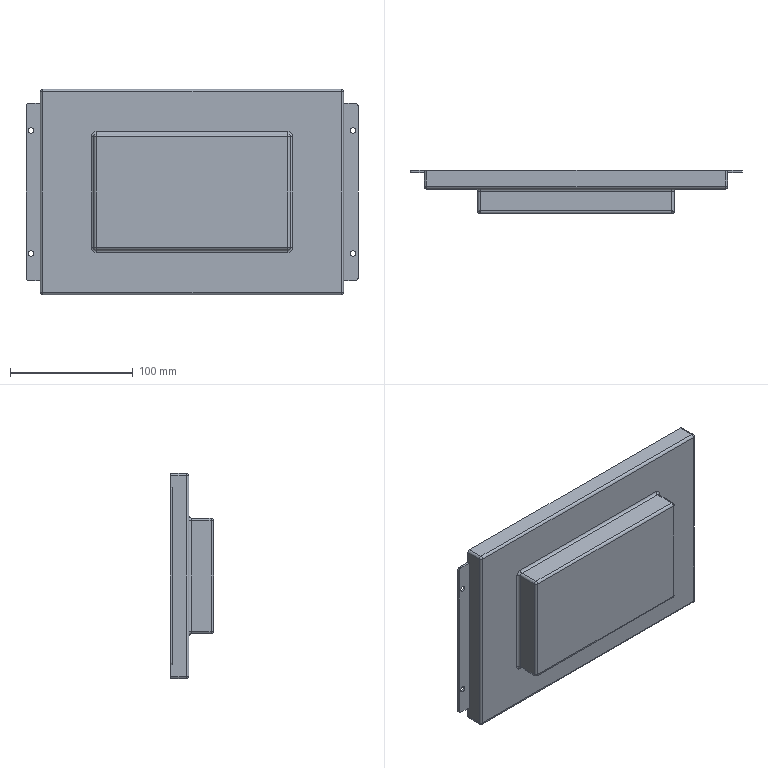Part | SolidWorks | features Fillet 3, ICE 3, Extrusion 1, HoleWzd 1 | 3 solids | 72 faces | box 270 x 35 x 167 mm | volume 892435 mm3 | cylinder 32 | plane 28 | sphere 8 | torus 4 | commonest cylinder face diameters 4 x24 4.5 x8